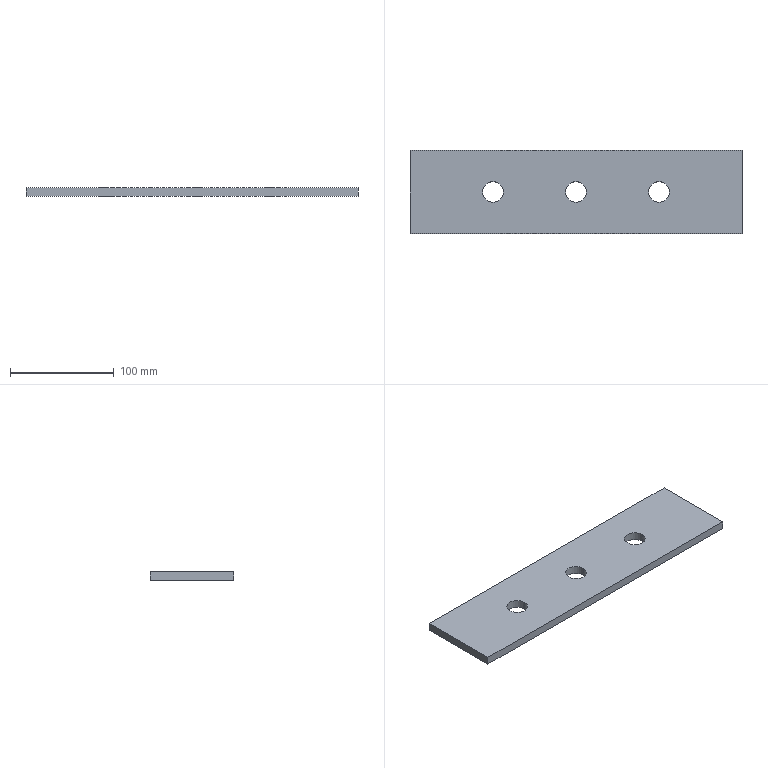Part | SolidWorks | features Extrusion 1, ICE 1 | 1 solid | 12 faces | box 320 x 80 x 8 mm | volume 197260 mm3 | cylinder 6 | plane 6 | commonest cylinder face diameters 20 x6
STEP:
#1=CARTESIAN_POINT('',(250.,40.,0.));
#2=VERTEX_POINT('',#1);
#3=CARTESIAN_POINT('',(230.,40.,0.));
#4=VERTEX_POINT('',#3);
#5=CARTESIAN_POINT('',(240.,40.,0.));
#6=DIRECTION('',(0.,0.,-1.));
#7=DIRECTION('',(-1.,0.,0.));
#8=AXIS2_PLACEMENT_3D('',#5,#6,#7);
#9=CIRCLE('',#8,10.);
#10=EDGE_CURVE('',#2,#4,#9,.T.);
#11=ORIENTED_EDGE('',*,*,#10,.T.);
#12=CARTESIAN_POINT('',(230.,40.,8.));
#13=VERTEX_POINT('',#12);
#14=CARTESIAN_POINT('',(230.,40.,-16.));
#15=DIRECTION('',(0.,0.,1.));
#16=VECTOR('',#15,1000.);
#17=LINE('',#14,#16);
#18=EDGE_CURVE('',#4,#13,#17,.T.);
#19=ORIENTED_EDGE('',*,*,#18,.T.);
#20=CARTESIAN_POINT('',(250.,40.,8.));
#21=VERTEX_POINT('',#20);
#22=CARTESIAN_POINT('',(240.,40.,8.));
#23=DIRECTION('',(0.,0.,1.));
#24=DIRECTION('',(1.,0.,0.));
#25=AXIS2_PLACEMENT_3D('',#22,#23,#24);
#26=CIRCLE('',#25,10.);
#27=EDGE_CURVE('',#13,#21,#26,.T.);
#28=ORIENTED_EDGE('',*,*,#27,.T.);
#29=CARTESIAN_POINT('',(250.,40.,-16.));
#30=DIRECTION('',(0.,0.,1.));
#31=VECTOR('',#30,1000.);
#32=LINE('',#29,#31);
#33=EDGE_CURVE('',#2,#21,#32,.T.);
#34=ORIENTED_EDGE('',*,*,#33,.F.);
#35=EDGE_LOOP('',(#11,#19,#28,#34));
#36=FACE_OUTER_BOUND('',#35,.T.);
#37=CARTESIAN_POINT('',(240.,40.,-16.));
#38=DIRECTION('',(0.,0.,1.));
#39=DIRECTION('',(1.,0.,0.));
#40=AXIS2_PLACEMENT_3D('',#37,#38,#39);
#41=CYLINDRICAL_SURFACE('',#40,10.);
#42=ADVANCED_FACE('',(#36),#41,.F.);
#43=CARTESIAN_POINT('',(170.,40.,0.));
#44=VERTEX_POINT('',#43);
#45=CARTESIAN_POINT('',(150.,40.,0.));
#46=VERTEX_POINT('',#45);
#47=CARTESIAN_POINT('',(160.,40.,0.));
#48=DIRECTION('',(0.,0.,-1.));
#49=DIRECTION('',(-1.,0.,0.));
#50=AXIS2_PLACEMENT_3D('',#47,#48,#49);
#51=CIRCLE('',#50,10.);
#52=EDGE_CURVE('',#44,#46,#51,.T.);
#53=ORIENTED_EDGE('',*,*,#52,.T.);
#54=CARTESIAN_POINT('',(150.,40.,8.));
#55=VERTEX_POINT('',#54);
#56=CARTESIAN_POINT('',(150.,40.,-16.));
#57=DIRECTION('',(0.,0.,1.));
#58=VECTOR('',#57,1000.);
#59=LINE('',#56,#58);
#60=EDGE_CURVE('',#46,#55,#59,.T.);
#61=ORIENTED_EDGE('',*,*,#60,.T.);
#62=CARTESIAN_POINT('',(170.,40.,8.));
#63=VERTEX_POINT('',#62);
#64=CARTESIAN_POINT('',(160.,40.,8.));
#65=DIRECTION('',(0.,0.,1.));
#66=DIRECTION('',(1.,0.,0.));
#67=AXIS2_PLACEMENT_3D('',#64,#65,#66);
#68=CIRCLE('',#67,10.);
#69=EDGE_CURVE('',#55,#63,#68,.T.);
#70=ORIENTED_EDGE('',*,*,#69,.T.);
#71=CARTESIAN_POINT('',(170.,40.,-16.));
#72=DIRECTION('',(0.,0.,1.));
#73=VECTOR('',#72,1000.);
#74=LINE('',#71,#73);
#75=EDGE_CURVE('',#44,#63,#74,.T.);
#76=ORIENTED_EDGE('',*,*,#75,.F.);
#77=EDGE_LOOP('',(#53,#61,#70,#76));
#78=FACE_OUTER_BOUND('',#77,.T.);
#79=CARTESIAN_POINT('',(160.,40.,-16.));
#80=DIRECTION('',(0.,0.,1.));
#81=DIRECTION('',(1.,0.,0.));
#82=AXIS2_PLACEMENT_3D('',#79,#80,#81);
#83=CYLINDRICAL_SURFACE('',#82,10.);
#84=ADVANCED_FACE('',(#78),#83,.F.);
#85=CARTESIAN_POINT('',(90.,40.,0.));
#86=VERTEX_POINT('',#85);
#87=CARTESIAN_POINT('',(70.,40.,0.));
#88=VERTEX_POINT('',#87);
#89=CARTESIAN_POINT('',(80.,40.,0.));
#90=DIRECTION('',(0.,0.,-1.));
#91=DIRECTION('',(-1.,0.,0.));
#92=AXIS2_PLACEMENT_3D('',#89,#90,#91);
#93=CIRCLE('',#92,10.);
#94=EDGE_CURVE('',#86,#88,#93,.T.);
#95=ORIENTED_EDGE('',*,*,#94,.T.);
#96=CARTESIAN_POINT('',(70.,40.,8.));
#97=VERTEX_POINT('',#96);
#98=CARTESIAN_POINT('',(70.,40.,-16.));
#99=DIRECTION('',(0.,0.,1.));
#100=VECTOR('',#99,1000.);
#101=LINE('',#98,#100);
#102=EDGE_CURVE('',#88,#97,#101,.T.);
#103=ORIENTED_EDGE('',*,*,#102,.T.);
#104=CARTESIAN_POINT('',(90.,40.,8.));
#105=VERTEX_POINT('',#104);
#106=CARTESIAN_POINT('',(80.,40.,8.));
#107=DIRECTION('',(0.,0.,1.));
#108=DIRECTION('',(1.,0.,0.));
#109=AXIS2_PLACEMENT_3D('',#106,#107,#108);
#110=CIRCLE('',#109,10.);
#111=EDGE_CURVE('',#97,#105,#110,.T.);
#112=ORIENTED_EDGE('',*,*,#111,.T.);
#113=CARTESIAN_POINT('',(90.,40.,-16.));
#114=DIRECTION('',(0.,0.,1.));
#115=VECTOR('',#114,1000.);
#116=LINE('',#113,#115);
#117=EDGE_CURVE('',#86,#105,#116,.T.);
#118=ORIENTED_EDGE('',*,*,#117,.F.);
#119=EDGE_LOOP('',(#95,#103,#112,#118));
#120=FACE_OUTER_BOUND('',#119,.T.);
#121=CARTESIAN_POINT('',(80.,40.,-16.));
#122=DIRECTION('',(0.,0.,1.));
#123=DIRECTION('',(1.,0.,0.));
#124=AXIS2_PLACEMENT_3D('',#121,#122,#123);
#125=CYLINDRICAL_SURFACE('',#124,10.);
#126=ADVANCED_FACE('',(#120),#125,.F.);
#127=CARTESIAN_POINT('',(0.,0.,0.));
#128=VERTEX_POINT('',#127);
#129=CARTESIAN_POINT('',(320.,0.,0.));
#130=VERTEX_POINT('',#129);
#131=CARTESIAN_POINT('',(320.,0.,0.));
#132=DIRECTION('',(1.,0.,0.));
#133=VECTOR('',#132,1000.);
#134=LINE('',#131,#133);
#135=EDGE_CURVE('',#128,#130,#134,.T.);
#136=ORIENTED_EDGE('',*,*,#135,.T.);
#137=CARTESIAN_POINT('',(320.,0.,8.));
#138=VERTEX_POINT('',#137);
#139=CARTESIAN_POINT('',(320.,0.,8.));
#140=DIRECTION('',(0.,0.,-1.));
#141=VECTOR('',#140,1000.);
#142=LINE('',#139,#141);
#143=EDGE_CURVE('',#138,#130,#142,.T.);
#144=ORIENTED_EDGE('',*,*,#143,.F.);
#145=CARTESIAN_POINT('',(0.,0.,8.));
#146=VERTEX_POINT('',#145);
#147=CARTESIAN_POINT('',(320.,0.,8.));
#148=DIRECTION('',(1.,0.,0.));
#149=VECTOR('',#148,1000.);
#150=LINE('',#147,#149);
#151=EDGE_CURVE('',#146,#138,#150,.T.);
#152=ORIENTED_EDGE('',*,*,#151,.F.);
#153=CARTESIAN_POINT('',(0.,0.,8.));
#154=DIRECTION('',(0.,0.,-1.));
#155=VECTOR('',#154,1000.);
#156=LINE('',#153,#155);
#157=EDGE_CURVE('',#146,#128,#156,.T.);
#158=ORIENTED_EDGE('',*,*,#157,.T.);
#159=EDGE_LOOP('',(#136,#144,#152,#158));
#160=FACE_OUTER_BOUND('',#159,.T.);
#161=CARTESIAN_POINT('',(320.,0.,8.));
#162=DIRECTION('',(0.,1.,0.));
#163=DIRECTION('',(0.,0.,1.));
#164=AXIS2_PLACEMENT_3D('',#161,#162,#163);
#165=PLANE('',#164);
#166=ADVANCED_FACE('',(#160),#165,.F.);
#167=CARTESIAN_POINT('',(320.,80.,0.));
#168=VERTEX_POINT('',#167);
#169=CARTESIAN_POINT('',(320.,80.,0.));
#170=DIRECTION('',(0.,1.,0.));
#171=VECTOR('',#170,1000.);
#172=LINE('',#169,#171);
#173=EDGE_CURVE('',#130,#168,#172,.T.);
#174=ORIENTED_EDGE('',*,*,#173,.T.);
#175=CARTESIAN_POINT('',(320.,80.,8.));
#176=VERTEX_POINT('',#175);
#177=CARTESIAN_POINT('',(320.,80.,8.));
#178=DIRECTION('',(0.,0.,-1.));
#179=VECTOR('',#178,1000.);
#180=LINE('',#177,#179);
#181=EDGE_CURVE('',#176,#168,#180,.T.);
#182=ORIENTED_EDGE('',*,*,#181,.F.);
#183=CARTESIAN_POINT('',(320.,80.,8.));
#184=DIRECTION('',(0.,1.,0.));
#185=VECTOR('',#184,1000.);
#186=LINE('',#183,#185);
#187=EDGE_CURVE('',#138,#176,#186,.T.);
#188=ORIENTED_EDGE('',*,*,#187,.F.);
#189=ORIENTED_EDGE('',*,*,#143,.T.);
#190=EDGE_LOOP('',(#174,#182,#188,#189));
#191=FACE_OUTER_BOUND('',#190,.T.);
#192=CARTESIAN_POINT('',(320.,80.,8.));
#193=DIRECTION('',(-1.,0.,0.));
#194=DIRECTION('',(0.,0.,1.));
#195=AXIS2_PLACEMENT_3D('',#192,#193,#194);
#196=PLANE('',#195);
#197=ADVANCED_FACE('',(#191),#196,.F.);
#198=CARTESIAN_POINT('',(0.,80.,0.));
#199=VERTEX_POINT('',#198);
#200=CARTESIAN_POINT('',(0.,80.,0.));
#201=DIRECTION('',(-1.,0.,0.));
#202=VECTOR('',#201,1000.);
#203=LINE('',#200,#202);
#204=EDGE_CURVE('',#168,#199,#203,.T.);
#205=ORIENTED_EDGE('',*,*,#204,.T.);
#206=CARTESIAN_POINT('',(0.,80.,8.));
#207=VERTEX_POINT('',#206);
#208=CARTESIAN_POINT('',(0.,80.,8.));
#209=DIRECTION('',(0.,0.,-1.));
#210=VECTOR('',#209,1000.);
#211=LINE('',#208,#210);
#212=EDGE_CURVE('',#207,#199,#211,.T.);
#213=ORIENTED_EDGE('',*,*,#212,.F.);
#214=CARTESIAN_POINT('',(310.,80.,8.));
#215=DIRECTION('',(-1.,0.,0.));
#216=VECTOR('',#215,1000.);
#217=LINE('',#214,#216);
#218=EDGE_CURVE('',#176,#207,#217,.T.);
#219=ORIENTED_EDGE('',*,*,#218,.F.);
#220=ORIENTED_EDGE('',*,*,#181,.T.);
#221=EDGE_LOOP('',(#205,#213,#219,#220));
#222=FACE_OUTER_BOUND('',#221,.T.);
#223=CARTESIAN_POINT('',(0.,80.,8.));
#224=DIRECTION('',(0.,-1.,0.));
#225=DIRECTION('',(0.,0.,-1.));
#226=AXIS2_PLACEMENT_3D('',#223,#224,#225);
#227=PLANE('',#226);
#228=ADVANCED_FACE('',(#222),#227,.F.);
#229=CARTESIAN_POINT('',(0.,0.,0.));
#230=DIRECTION('',(0.,-1.,0.));
#231=VECTOR('',#230,1000.);
#232=LINE('',#229,#231);
#233=EDGE_CURVE('',#199,#128,#232,.T.);
#234=ORIENTED_EDGE('',*,*,#233,.T.);
#235=ORIENTED_EDGE('',*,*,#157,.F.);
#236=CARTESIAN_POINT('',(0.,0.,8.));
#237=DIRECTION('',(0.,-1.,0.));
#238=VECTOR('',#237,1000.);
#239=LINE('',#236,#238);
#240=EDGE_CURVE('',#207,#146,#239,.T.);
#241=ORIENTED_EDGE('',*,*,#240,.F.);
#242=ORIENTED_EDGE('',*,*,#212,.T.);
#243=EDGE_LOOP('',(#234,#235,#241,#242));
#244=FACE_OUTER_BOUND('',#243,.T.);
#245=CARTESIAN_POINT('',(0.,0.,8.));
#246=DIRECTION('',(1.,0.,0.));
#247=DIRECTION('',(0.,0.,-1.));
#248=AXIS2_PLACEMENT_3D('',#245,#246,#247);
#249=PLANE('',#248);
#250=ADVANCED_FACE('',(#244),#249,.F.);
#251=CARTESIAN_POINT('',(240.,40.,8.));
#252=DIRECTION('',(0.,0.,1.));
#253=DIRECTION('',(1.,0.,0.));
#254=AXIS2_PLACEMENT_3D('',#251,#252,#253);
#255=CIRCLE('',#254,10.);
#256=EDGE_CURVE('',#21,#13,#255,.T.);
#257=ORIENTED_EDGE('',*,*,#256,.F.);
#258=ORIENTED_EDGE('',*,*,#27,.F.);
#259=EDGE_LOOP('',(#257,#258));
#260=FACE_BOUND('',#259,.T.);
#261=CARTESIAN_POINT('',(160.,40.,8.));
#262=DIRECTION('',(0.,0.,1.));
#263=DIRECTION('',(1.,0.,0.));
#264=AXIS2_PLACEMENT_3D('',#261,#262,#263);
#265=CIRCLE('',#264,10.);
#266=EDGE_CURVE('',#63,#55,#265,.T.);
#267=ORIENTED_EDGE('',*,*,#266,.F.);
#268=ORIENTED_EDGE('',*,*,#69,.F.);
#269=EDGE_LOOP('',(#267,#268));
#270=FACE_BOUND('',#269,.T.);
#271=CARTESIAN_POINT('',(80.,40.,8.));
#272=DIRECTION('',(0.,0.,1.));
#273=DIRECTION('',(1.,0.,0.));
#274=AXIS2_PLACEMENT_3D('',#271,#272,#273);
#275=CIRCLE('',#274,10.);
#276=EDGE_CURVE('',#105,#97,#275,.T.);
#277=ORIENTED_EDGE('',*,*,#276,.F.);
#278=ORIENTED_EDGE('',*,*,#111,.F.);
#279=EDGE_LOOP('',(#277,#278));
#280=FACE_BOUND('',#279,.T.);
#281=ORIENTED_EDGE('',*,*,#151,.T.);
#282=ORIENTED_EDGE('',*,*,#187,.T.);
#283=ORIENTED_EDGE('',*,*,#218,.T.);
#284=ORIENTED_EDGE('',*,*,#240,.T.);
#285=EDGE_LOOP('',(#281,#282,#283,#284));
#286=FACE_OUTER_BOUND('',#285,.T.);
#287=CARTESIAN_POINT('',(0.,0.,8.));
#288=DIRECTION('',(0.,0.,-1.));
#289=DIRECTION('',(-1.,0.,0.));
#290=AXIS2_PLACEMENT_3D('',#287,#288,#289);
#291=PLANE('',#290);
#292=ADVANCED_FACE('',(#260,#270,#280,#286),#291,.F.);
#293=ORIENTED_EDGE('',*,*,#10,.F.);
#294=CARTESIAN_POINT('',(240.,40.,0.));
#295=DIRECTION('',(0.,0.,-1.));
#296=DIRECTION('',(-1.,0.,0.));
#297=AXIS2_PLACEMENT_3D('',#294,#295,#296);
#298=CIRCLE('',#297,10.);
#299=EDGE_CURVE('',#4,#2,#298,.T.);
#300=ORIENTED_EDGE('',*,*,#299,.F.);
#301=EDGE_LOOP('',(#293,#300));
#302=FACE_BOUND('',#301,.T.);
#303=ORIENTED_EDGE('',*,*,#52,.F.);
#304=CARTESIAN_POINT('',(160.,40.,0.));
#305=DIRECTION('',(0.,0.,-1.));
#306=DIRECTION('',(-1.,0.,0.));
#307=AXIS2_PLACEMENT_3D('',#304,#305,#306);
#308=CIRCLE('',#307,10.);
#309=EDGE_CURVE('',#46,#44,#308,.T.);
#310=ORIENTED_EDGE('',*,*,#309,.F.);
#311=EDGE_LOOP('',(#303,#310));
#312=FACE_BOUND('',#311,.T.);
#313=ORIENTED_EDGE('',*,*,#94,.F.);
#314=CARTESIAN_POINT('',(80.,40.,0.));
#315=DIRECTION('',(0.,0.,-1.));
#316=DIRECTION('',(-1.,0.,0.));
#317=AXIS2_PLACEMENT_3D('',#314,#315,#316);
#318=CIRCLE('',#317,10.);
#319=EDGE_CURVE('',#88,#86,#318,.T.);
#320=ORIENTED_EDGE('',*,*,#319,.F.);
#321=EDGE_LOOP('',(#313,#320));
#322=FACE_BOUND('',#321,.T.);
#323=ORIENTED_EDGE('',*,*,#135,.F.);
#324=ORIENTED_EDGE('',*,*,#233,.F.);
#325=ORIENTED_EDGE('',*,*,#204,.F.);
#326=ORIENTED_EDGE('',*,*,#173,.F.);
#327=EDGE_LOOP('',(#323,#324,#325,#326));
#328=FACE_OUTER_BOUND('',#327,.T.);
#329=CARTESIAN_POINT('',(0.,0.,0.));
#330=DIRECTION('',(0.,0.,-1.));
#331=DIRECTION('',(-1.,0.,0.));
#332=AXIS2_PLACEMENT_3D('',#329,#330,#331);
#333=PLANE('',#332);
#334=ADVANCED_FACE('',(#302,#312,#322,#328),#333,.T.);
#335=ORIENTED_EDGE('',*,*,#102,.F.);
#336=ORIENTED_EDGE('',*,*,#319,.T.);
#337=ORIENTED_EDGE('',*,*,#117,.T.);
#338=ORIENTED_EDGE('',*,*,#276,.T.);
#339=EDGE_LOOP('',(#335,#336,#337,#338));
#340=FACE_OUTER_BOUND('',#339,.T.);
#341=CARTESIAN_POINT('',(80.,40.,-16.));
#342=DIRECTION('',(0.,0.,1.));
#343=DIRECTION('',(1.,0.,0.));
#344=AXIS2_PLACEMENT_3D('',#341,#342,#343);
#345=CYLINDRICAL_SURFACE('',#344,10.);
#346=ADVANCED_FACE('',(#340),#345,.F.);
#347=ORIENTED_EDGE('',*,*,#60,.F.);
#348=ORIENTED_EDGE('',*,*,#309,.T.);
#349=ORIENTED_EDGE('',*,*,#75,.T.);
#350=ORIENTED_EDGE('',*,*,#266,.T.);
#351=EDGE_LOOP('',(#347,#348,#349,#350));
#352=FACE_OUTER_BOUND('',#351,.T.);
#353=CARTESIAN_POINT('',(160.,40.,-16.));
#354=DIRECTION('',(0.,0.,1.));
#355=DIRECTION('',(1.,0.,0.));
#356=AXIS2_PLACEMENT_3D('',#353,#354,#355);
#357=CYLINDRICAL_SURFACE('',#356,10.);
#358=ADVANCED_FACE('',(#352),#357,.F.);
#359=ORIENTED_EDGE('',*,*,#18,.F.);
#360=ORIENTED_EDGE('',*,*,#299,.T.);
#361=ORIENTED_EDGE('',*,*,#33,.T.);
#362=ORIENTED_EDGE('',*,*,#256,.T.);
#363=EDGE_LOOP('',(#359,#360,#361,#362));
#364=FACE_OUTER_BOUND('',#363,.T.);
#365=CARTESIAN_POINT('',(240.,40.,-16.));
#366=DIRECTION('',(0.,0.,1.));
#367=DIRECTION('',(1.,0.,0.));
#368=AXIS2_PLACEMENT_3D('',#365,#366,#367);
#369=CYLINDRICAL_SURFACE('',#368,10.);
#370=ADVANCED_FACE('',(#364),#369,.F.);
#371=CLOSED_SHELL('',(#42,#84,#126,#166,#197,#228,#250,#292,#334,#346,#358,#370));
#372=MANIFOLD_SOLID_BREP('',#371);
#373=CARTESIAN_POINT('',(0.,0.,0.));
#374=DIRECTION('',(0.,0.,1.));
#375=DIRECTION('',(1.,0.,0.));
#376=AXIS2_PLACEMENT_3D('',#373,#374,#375);
#377=(LENGTH_UNIT()NAMED_UNIT(*)SI_UNIT(.MILLI.,.METRE.));
#378=UNCERTAINTY_MEASURE_WITH_UNIT(LENGTH_MEASURE(0.00001),#377,'','');
#379=(NAMED_UNIT(*)PLANE_ANGLE_UNIT()SI_UNIT($,.RADIAN.));
#380=(NAMED_UNIT(*)SI_UNIT($,.STERADIAN.)SOLID_ANGLE_UNIT());
#381=(GEOMETRIC_REPRESENTATION_CONTEXT(3)GLOBAL_UNCERTAINTY_ASSIGNED_CONTEXT((#378))GLOBAL_UNIT_ASSIGNED_CONTEXT((#377,#379,#380))REPRESENTATION_CONTEXT('',''));
#382=ADVANCED_BREP_SHAPE_REPRESENTATION('',(#372,#376),#381);